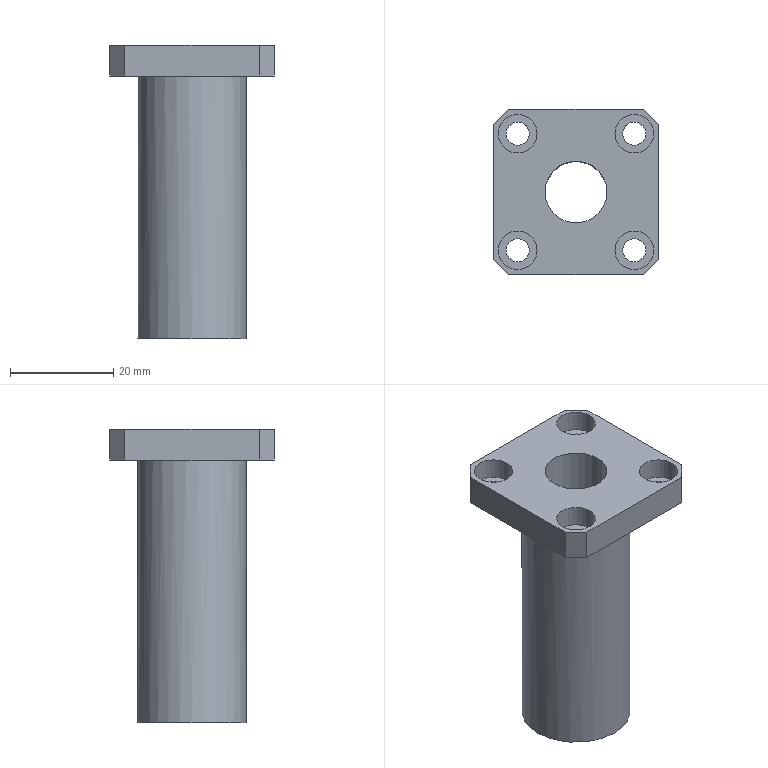Part | STEP file | YBQDJ-PD-11 | 1 solid | 25 faces | box 32 x 32 x 57 mm | volume 16408 mm3 | plane 15 | cylinder 10 | commonest cylinder face diameters 4.5 x4 7.5 x4 12 x1 21 x1